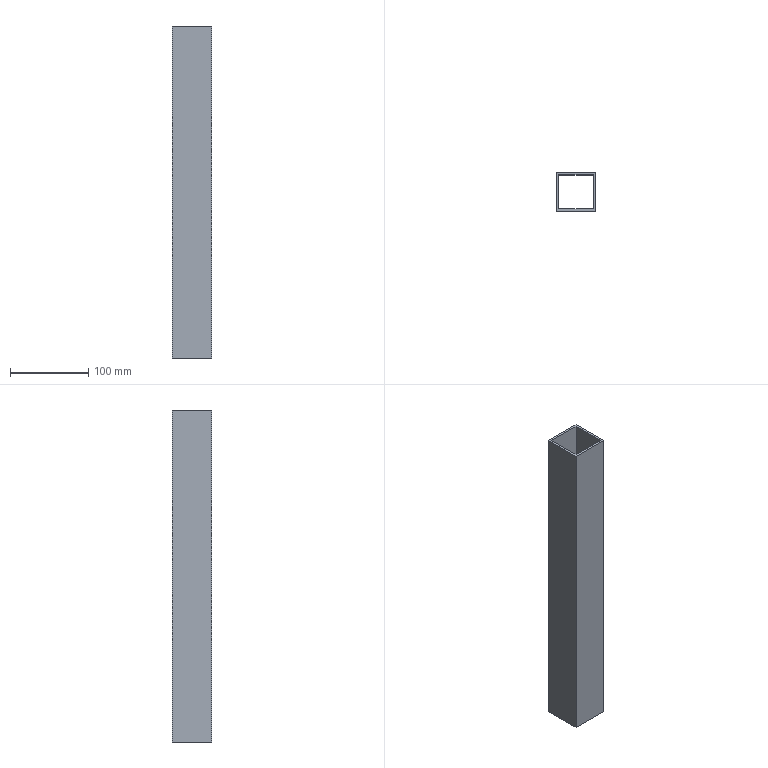Part | SolidWorks | features Cut 1, Extrusion 1, ICE 1 | 1 solid | 10 faces | box 50 x 50 x 425 mm | volume 239700 mm3 | plane 10
STEP:
#1=CARTESIAN_POINT('',(0.,50.,400.));
#2=VERTEX_POINT('',#1);
#3=CARTESIAN_POINT('',(0.,50.,-25.));
#4=VERTEX_POINT('',#3);
#5=CARTESIAN_POINT('',(0.,50.,400.));
#6=DIRECTION('',(0.,0.,-1.));
#7=VECTOR('',#6,1000.);
#8=LINE('',#5,#7);
#9=EDGE_CURVE('',#2,#4,#8,.T.);
#10=ORIENTED_EDGE('',*,*,#9,.T.);
#11=CARTESIAN_POINT('',(0.,0.,-25.));
#12=VERTEX_POINT('',#11);
#13=CARTESIAN_POINT('',(0.,0.,-25.));
#14=DIRECTION('',(0.,1.,0.));
#15=VECTOR('',#14,1000.);
#16=LINE('',#13,#15);
#17=EDGE_CURVE('',#12,#4,#16,.T.);
#18=ORIENTED_EDGE('',*,*,#17,.F.);
#19=CARTESIAN_POINT('',(0.,0.,400.));
#20=VERTEX_POINT('',#19);
#21=CARTESIAN_POINT('',(0.,0.,400.));
#22=DIRECTION('',(0.,0.,-1.));
#23=VECTOR('',#22,1000.);
#24=LINE('',#21,#23);
#25=EDGE_CURVE('',#20,#12,#24,.T.);
#26=ORIENTED_EDGE('',*,*,#25,.F.);
#27=CARTESIAN_POINT('',(0.,50.,400.));
#28=DIRECTION('',(0.,-1.,0.));
#29=VECTOR('',#28,1000.);
#30=LINE('',#27,#29);
#31=EDGE_CURVE('',#2,#20,#30,.T.);
#32=ORIENTED_EDGE('',*,*,#31,.F.);
#33=EDGE_LOOP('',(#10,#18,#26,#32));
#34=FACE_OUTER_BOUND('',#33,.T.);
#35=CARTESIAN_POINT('',(0.,50.,400.));
#36=DIRECTION('',(1.,0.,0.));
#37=DIRECTION('',(0.,0.,-1.));
#38=AXIS2_PLACEMENT_3D('',#35,#36,#37);
#39=PLANE('',#38);
#40=ADVANCED_FACE('',(#34),#39,.F.);
#41=ORIENTED_EDGE('',*,*,#25,.T.);
#42=CARTESIAN_POINT('',(50.,0.,-25.));
#43=VERTEX_POINT('',#42);
#44=CARTESIAN_POINT('',(50.,0.,-25.));
#45=DIRECTION('',(-1.,0.,0.));
#46=VECTOR('',#45,1000.);
#47=LINE('',#44,#46);
#48=EDGE_CURVE('',#43,#12,#47,.T.);
#49=ORIENTED_EDGE('',*,*,#48,.F.);
#50=CARTESIAN_POINT('',(50.,0.,400.));
#51=VERTEX_POINT('',#50);
#52=CARTESIAN_POINT('',(50.,0.,400.));
#53=DIRECTION('',(0.,0.,-1.));
#54=VECTOR('',#53,1000.);
#55=LINE('',#52,#54);
#56=EDGE_CURVE('',#51,#43,#55,.T.);
#57=ORIENTED_EDGE('',*,*,#56,.F.);
#58=CARTESIAN_POINT('',(0.,0.,400.));
#59=DIRECTION('',(1.,0.,0.));
#60=VECTOR('',#59,1000.);
#61=LINE('',#58,#60);
#62=EDGE_CURVE('',#20,#51,#61,.T.);
#63=ORIENTED_EDGE('',*,*,#62,.F.);
#64=EDGE_LOOP('',(#41,#49,#57,#63));
#65=FACE_OUTER_BOUND('',#64,.T.);
#66=CARTESIAN_POINT('',(0.,0.,400.));
#67=DIRECTION('',(0.,1.,0.));
#68=DIRECTION('',(0.,0.,1.));
#69=AXIS2_PLACEMENT_3D('',#66,#67,#68);
#70=PLANE('',#69);
#71=ADVANCED_FACE('',(#65),#70,.F.);
#72=ORIENTED_EDGE('',*,*,#56,.T.);
#73=CARTESIAN_POINT('',(50.,50.,-25.));
#74=VERTEX_POINT('',#73);
#75=CARTESIAN_POINT('',(50.,50.,-25.));
#76=DIRECTION('',(0.,-1.,0.));
#77=VECTOR('',#76,1000.);
#78=LINE('',#75,#77);
#79=EDGE_CURVE('',#74,#43,#78,.T.);
#80=ORIENTED_EDGE('',*,*,#79,.F.);
#81=CARTESIAN_POINT('',(50.,50.,400.));
#82=VERTEX_POINT('',#81);
#83=CARTESIAN_POINT('',(50.,50.,400.));
#84=DIRECTION('',(0.,0.,-1.));
#85=VECTOR('',#84,1000.);
#86=LINE('',#83,#85);
#87=EDGE_CURVE('',#82,#74,#86,.T.);
#88=ORIENTED_EDGE('',*,*,#87,.F.);
#89=CARTESIAN_POINT('',(50.,0.,400.));
#90=DIRECTION('',(0.,1.,0.));
#91=VECTOR('',#90,1000.);
#92=LINE('',#89,#91);
#93=EDGE_CURVE('',#51,#82,#92,.T.);
#94=ORIENTED_EDGE('',*,*,#93,.F.);
#95=EDGE_LOOP('',(#72,#80,#88,#94));
#96=FACE_OUTER_BOUND('',#95,.T.);
#97=CARTESIAN_POINT('',(50.,0.,400.));
#98=DIRECTION('',(-1.,0.,0.));
#99=DIRECTION('',(0.,0.,1.));
#100=AXIS2_PLACEMENT_3D('',#97,#98,#99);
#101=PLANE('',#100);
#102=ADVANCED_FACE('',(#96),#101,.F.);
#103=ORIENTED_EDGE('',*,*,#87,.T.);
#104=CARTESIAN_POINT('',(0.,50.,-25.));
#105=DIRECTION('',(1.,0.,0.));
#106=VECTOR('',#105,1000.);
#107=LINE('',#104,#106);
#108=EDGE_CURVE('',#4,#74,#107,.T.);
#109=ORIENTED_EDGE('',*,*,#108,.F.);
#110=ORIENTED_EDGE('',*,*,#9,.F.);
#111=CARTESIAN_POINT('',(50.,50.,400.));
#112=DIRECTION('',(-1.,0.,0.));
#113=VECTOR('',#112,1000.);
#114=LINE('',#111,#113);
#115=EDGE_CURVE('',#82,#2,#114,.T.);
#116=ORIENTED_EDGE('',*,*,#115,.F.);
#117=EDGE_LOOP('',(#103,#109,#110,#116));
#118=FACE_OUTER_BOUND('',#117,.T.);
#119=CARTESIAN_POINT('',(50.,50.,400.));
#120=DIRECTION('',(0.,-1.,0.));
#121=DIRECTION('',(0.,0.,-1.));
#122=AXIS2_PLACEMENT_3D('',#119,#120,#121);
#123=PLANE('',#122);
#124=ADVANCED_FACE('',(#118),#123,.F.);
#125=CARTESIAN_POINT('',(3.,3.,400.));
#126=VERTEX_POINT('',#125);
#127=CARTESIAN_POINT('',(3.,3.,-25.));
#128=VERTEX_POINT('',#127);
#129=CARTESIAN_POINT('',(3.,3.,400.));
#130=DIRECTION('',(0.,0.,-1.));
#131=VECTOR('',#130,1000.);
#132=LINE('',#129,#131);
#133=EDGE_CURVE('',#126,#128,#132,.T.);
#134=ORIENTED_EDGE('',*,*,#133,.T.);
#135=CARTESIAN_POINT('',(3.,47.,-25.));
#136=VERTEX_POINT('',#135);
#137=CARTESIAN_POINT('',(3.,3.,-25.));
#138=DIRECTION('',(0.,1.,0.));
#139=VECTOR('',#138,1000.);
#140=LINE('',#137,#139);
#141=EDGE_CURVE('',#128,#136,#140,.T.);
#142=ORIENTED_EDGE('',*,*,#141,.T.);
#143=CARTESIAN_POINT('',(3.,47.,400.));
#144=VERTEX_POINT('',#143);
#145=CARTESIAN_POINT('',(3.,47.,400.));
#146=DIRECTION('',(0.,0.,-1.));
#147=VECTOR('',#146,1000.);
#148=LINE('',#145,#147);
#149=EDGE_CURVE('',#144,#136,#148,.T.);
#150=ORIENTED_EDGE('',*,*,#149,.F.);
#151=CARTESIAN_POINT('',(3.,47.,400.));
#152=DIRECTION('',(0.,-1.,0.));
#153=VECTOR('',#152,1000.);
#154=LINE('',#151,#153);
#155=EDGE_CURVE('',#144,#126,#154,.T.);
#156=ORIENTED_EDGE('',*,*,#155,.T.);
#157=EDGE_LOOP('',(#134,#142,#150,#156));
#158=FACE_OUTER_BOUND('',#157,.T.);
#159=CARTESIAN_POINT('',(3.,47.,400.));
#160=DIRECTION('',(1.,0.,0.));
#161=DIRECTION('',(0.,0.,-1.));
#162=AXIS2_PLACEMENT_3D('',#159,#160,#161);
#163=PLANE('',#162);
#164=ADVANCED_FACE('',(#158),#163,.T.);
#165=CARTESIAN_POINT('',(47.,3.,400.));
#166=VERTEX_POINT('',#165);
#167=CARTESIAN_POINT('',(47.,3.,-25.));
#168=VERTEX_POINT('',#167);
#169=CARTESIAN_POINT('',(47.,3.,400.));
#170=DIRECTION('',(0.,0.,-1.));
#171=VECTOR('',#170,1000.);
#172=LINE('',#169,#171);
#173=EDGE_CURVE('',#166,#168,#172,.T.);
#174=ORIENTED_EDGE('',*,*,#173,.T.);
#175=CARTESIAN_POINT('',(47.,3.,-25.));
#176=DIRECTION('',(-1.,0.,0.));
#177=VECTOR('',#176,1000.);
#178=LINE('',#175,#177);
#179=EDGE_CURVE('',#168,#128,#178,.T.);
#180=ORIENTED_EDGE('',*,*,#179,.T.);
#181=ORIENTED_EDGE('',*,*,#133,.F.);
#182=CARTESIAN_POINT('',(3.,3.,400.));
#183=DIRECTION('',(1.,0.,0.));
#184=VECTOR('',#183,1000.);
#185=LINE('',#182,#184);
#186=EDGE_CURVE('',#126,#166,#185,.T.);
#187=ORIENTED_EDGE('',*,*,#186,.T.);
#188=EDGE_LOOP('',(#174,#180,#181,#187));
#189=FACE_OUTER_BOUND('',#188,.T.);
#190=CARTESIAN_POINT('',(3.,3.,400.));
#191=DIRECTION('',(0.,1.,0.));
#192=DIRECTION('',(0.,0.,1.));
#193=AXIS2_PLACEMENT_3D('',#190,#191,#192);
#194=PLANE('',#193);
#195=ADVANCED_FACE('',(#189),#194,.T.);
#196=CARTESIAN_POINT('',(47.,47.,400.));
#197=VERTEX_POINT('',#196);
#198=CARTESIAN_POINT('',(47.,47.,-25.));
#199=VERTEX_POINT('',#198);
#200=CARTESIAN_POINT('',(47.,47.,400.));
#201=DIRECTION('',(0.,0.,-1.));
#202=VECTOR('',#201,1000.);
#203=LINE('',#200,#202);
#204=EDGE_CURVE('',#197,#199,#203,.T.);
#205=ORIENTED_EDGE('',*,*,#204,.T.);
#206=CARTESIAN_POINT('',(47.,47.,-25.));
#207=DIRECTION('',(0.,-1.,0.));
#208=VECTOR('',#207,1000.);
#209=LINE('',#206,#208);
#210=EDGE_CURVE('',#199,#168,#209,.T.);
#211=ORIENTED_EDGE('',*,*,#210,.T.);
#212=ORIENTED_EDGE('',*,*,#173,.F.);
#213=CARTESIAN_POINT('',(47.,3.,400.));
#214=DIRECTION('',(0.,1.,0.));
#215=VECTOR('',#214,1000.);
#216=LINE('',#213,#215);
#217=EDGE_CURVE('',#166,#197,#216,.T.);
#218=ORIENTED_EDGE('',*,*,#217,.T.);
#219=EDGE_LOOP('',(#205,#211,#212,#218));
#220=FACE_OUTER_BOUND('',#219,.T.);
#221=CARTESIAN_POINT('',(47.,3.,400.));
#222=DIRECTION('',(-1.,0.,0.));
#223=DIRECTION('',(0.,0.,1.));
#224=AXIS2_PLACEMENT_3D('',#221,#222,#223);
#225=PLANE('',#224);
#226=ADVANCED_FACE('',(#220),#225,.T.);
#227=ORIENTED_EDGE('',*,*,#149,.T.);
#228=CARTESIAN_POINT('',(3.,47.,-25.));
#229=DIRECTION('',(1.,0.,0.));
#230=VECTOR('',#229,1000.);
#231=LINE('',#228,#230);
#232=EDGE_CURVE('',#136,#199,#231,.T.);
#233=ORIENTED_EDGE('',*,*,#232,.T.);
#234=ORIENTED_EDGE('',*,*,#204,.F.);
#235=CARTESIAN_POINT('',(47.,47.,400.));
#236=DIRECTION('',(-1.,0.,0.));
#237=VECTOR('',#236,1000.);
#238=LINE('',#235,#237);
#239=EDGE_CURVE('',#197,#144,#238,.T.);
#240=ORIENTED_EDGE('',*,*,#239,.T.);
#241=EDGE_LOOP('',(#227,#233,#234,#240));
#242=FACE_OUTER_BOUND('',#241,.T.);
#243=CARTESIAN_POINT('',(47.,47.,400.));
#244=DIRECTION('',(0.,-1.,0.));
#245=DIRECTION('',(0.,0.,-1.));
#246=AXIS2_PLACEMENT_3D('',#243,#244,#245);
#247=PLANE('',#246);
#248=ADVANCED_FACE('',(#242),#247,.T.);
#249=ORIENTED_EDGE('',*,*,#31,.T.);
#250=ORIENTED_EDGE('',*,*,#62,.T.);
#251=ORIENTED_EDGE('',*,*,#93,.T.);
#252=ORIENTED_EDGE('',*,*,#115,.T.);
#253=EDGE_LOOP('',(#249,#250,#251,#252));
#254=FACE_OUTER_BOUND('',#253,.T.);
#255=ORIENTED_EDGE('',*,*,#186,.F.);
#256=ORIENTED_EDGE('',*,*,#155,.F.);
#257=ORIENTED_EDGE('',*,*,#239,.F.);
#258=ORIENTED_EDGE('',*,*,#217,.F.);
#259=EDGE_LOOP('',(#255,#256,#257,#258));
#260=FACE_BOUND('',#259,.T.);
#261=CARTESIAN_POINT('',(0.,0.,400.));
#262=DIRECTION('',(0.,0.,1.));
#263=DIRECTION('',(1.,0.,0.));
#264=AXIS2_PLACEMENT_3D('',#261,#262,#263);
#265=PLANE('',#264);
#266=ADVANCED_FACE('',(#254,#260),#265,.T.);
#267=ORIENTED_EDGE('',*,*,#79,.T.);
#268=ORIENTED_EDGE('',*,*,#48,.T.);
#269=ORIENTED_EDGE('',*,*,#17,.T.);
#270=ORIENTED_EDGE('',*,*,#108,.T.);
#271=EDGE_LOOP('',(#267,#268,#269,#270));
#272=FACE_OUTER_BOUND('',#271,.T.);
#273=ORIENTED_EDGE('',*,*,#210,.F.);
#274=ORIENTED_EDGE('',*,*,#232,.F.);
#275=ORIENTED_EDGE('',*,*,#141,.F.);
#276=ORIENTED_EDGE('',*,*,#179,.F.);
#277=EDGE_LOOP('',(#273,#274,#275,#276));
#278=FACE_BOUND('',#277,.T.);
#279=CARTESIAN_POINT('',(0.,0.,-25.));
#280=DIRECTION('',(0.,0.,-1.));
#281=DIRECTION('',(-1.,0.,0.));
#282=AXIS2_PLACEMENT_3D('',#279,#280,#281);
#283=PLANE('',#282);
#284=ADVANCED_FACE('',(#272,#278),#283,.T.);
#285=CLOSED_SHELL('',(#40,#71,#102,#124,#164,#195,#226,#248,#266,#284));
#286=MANIFOLD_SOLID_BREP('',#285);
#287=CARTESIAN_POINT('',(0.,0.,0.));
#288=DIRECTION('',(0.,0.,1.));
#289=DIRECTION('',(1.,0.,0.));
#290=AXIS2_PLACEMENT_3D('',#287,#288,#289);
#291=(LENGTH_UNIT()NAMED_UNIT(*)SI_UNIT(.MILLI.,.METRE.));
#292=UNCERTAINTY_MEASURE_WITH_UNIT(LENGTH_MEASURE(0.00001),#291,'','');
#293=(NAMED_UNIT(*)PLANE_ANGLE_UNIT()SI_UNIT($,.RADIAN.));
#294=(NAMED_UNIT(*)SI_UNIT($,.STERADIAN.)SOLID_ANGLE_UNIT());
#295=(GEOMETRIC_REPRESENTATION_CONTEXT(3)GLOBAL_UNCERTAINTY_ASSIGNED_CONTEXT((#292))GLOBAL_UNIT_ASSIGNED_CONTEXT((#291,#293,#294))REPRESENTATION_CONTEXT('',''));
#296=ADVANCED_BREP_SHAPE_REPRESENTATION('',(#286,#290),#295);